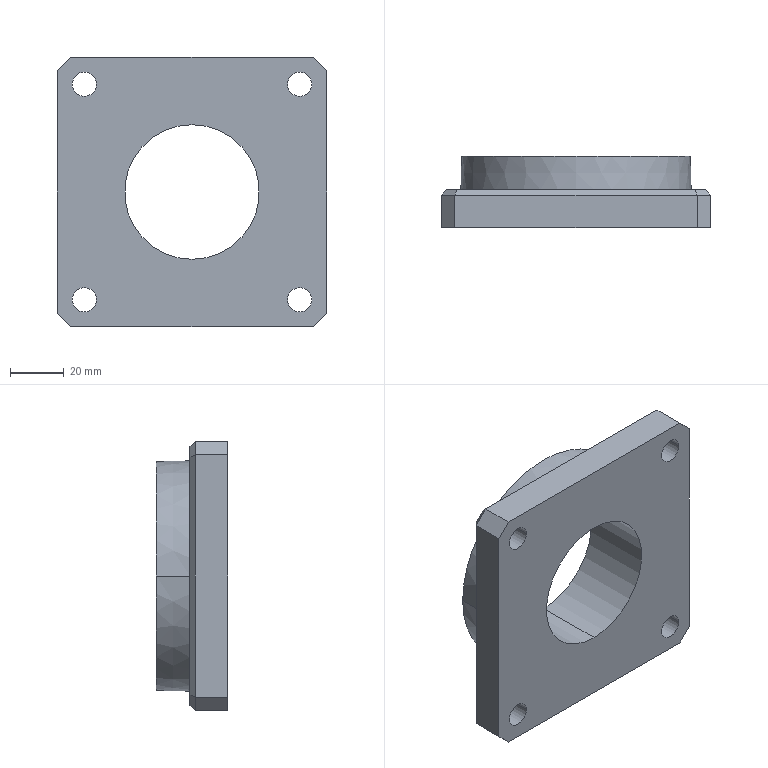Part | SolidWorks | features BaseBody 1 | 1 solid | 43 faces | box 100 x 26.5 x 100 mm | volume 151734 mm3 | plane 23 | cylinder 18 | cone 2 | commonest cylinder face diameters 9 x8 14 x8 50 x2
STEP:
#1=CARTESIAN_POINT('',(66.,42.,40.));
#2=VERTEX_POINT('',#1);
#3=CARTESIAN_POINT('',(80.,42.,40.));
#4=VERTEX_POINT('',#3);
#5=CARTESIAN_POINT('',(73.,42.,40.));
#6=DIRECTION('',(0.,1.,0.));
#7=DIRECTION('',(-1.,0.,0.));
#8=AXIS2_PLACEMENT_3D('',#5,#6,#7);
#9=CIRCLE('',#8,7.);
#10=EDGE_CURVE('',#2,#4,#9,.T.);
#11=ORIENTED_EDGE('',*,*,#10,.F.);
#12=CARTESIAN_POINT('',(66.,49.,40.));
#13=VERTEX_POINT('',#12);
#14=CARTESIAN_POINT('',(66.,49.,40.));
#15=DIRECTION('',(0.,1.,0.));
#16=VECTOR('',#15,1000.);
#17=LINE('',#14,#16);
#18=EDGE_CURVE('',#2,#13,#17,.T.);
#19=ORIENTED_EDGE('',*,*,#18,.T.);
#20=CARTESIAN_POINT('',(80.,49.,40.));
#21=VERTEX_POINT('',#20);
#22=CARTESIAN_POINT('',(73.,49.,40.));
#23=DIRECTION('',(0.,-1.,0.));
#24=DIRECTION('',(1.,0.,0.));
#25=AXIS2_PLACEMENT_3D('',#22,#23,#24);
#26=CIRCLE('',#25,7.);
#27=EDGE_CURVE('',#21,#13,#26,.T.);
#28=ORIENTED_EDGE('',*,*,#27,.F.);
#29=CARTESIAN_POINT('',(80.,49.,40.));
#30=DIRECTION('',(0.,1.,0.));
#31=VECTOR('',#30,1000.);
#32=LINE('',#29,#31);
#33=EDGE_CURVE('',#4,#21,#32,.T.);
#34=ORIENTED_EDGE('',*,*,#33,.F.);
#35=EDGE_LOOP('',(#11,#19,#28,#34));
#36=FACE_OUTER_BOUND('',#35,.T.);
#37=CARTESIAN_POINT('',(73.,49.,40.));
#38=DIRECTION('',(0.,1.,0.));
#39=DIRECTION('',(1.,0.,0.));
#40=AXIS2_PLACEMENT_3D('',#37,#38,#39);
#41=CYLINDRICAL_SURFACE('',#40,7.);
#42=ADVANCED_FACE('',(#36),#41,.F.);
#43=CARTESIAN_POINT('',(77.5,42.,40.));
#44=VERTEX_POINT('',#43);
#45=CARTESIAN_POINT('',(68.5,42.,40.));
#46=VERTEX_POINT('',#45);
#47=CARTESIAN_POINT('',(73.,42.,40.));
#48=DIRECTION('',(0.,-1.,0.));
#49=DIRECTION('',(-1.,0.,0.));
#50=AXIS2_PLACEMENT_3D('',#47,#48,#49);
#51=CIRCLE('',#50,4.5);
#52=EDGE_CURVE('',#44,#46,#51,.T.);
#53=ORIENTED_EDGE('',*,*,#52,.F.);
#54=CARTESIAN_POINT('',(77.5,35.,40.));
#55=VERTEX_POINT('',#54);
#56=CARTESIAN_POINT('',(77.5,35.,40.));
#57=DIRECTION('',(0.,-1.,0.));
#58=VECTOR('',#57,1000.);
#59=LINE('',#56,#58);
#60=EDGE_CURVE('',#44,#55,#59,.T.);
#61=ORIENTED_EDGE('',*,*,#60,.T.);
#62=CARTESIAN_POINT('',(68.5,35.,40.));
#63=VERTEX_POINT('',#62);
#64=CARTESIAN_POINT('',(73.,35.,40.));
#65=DIRECTION('',(0.,1.,0.));
#66=DIRECTION('',(1.,0.,0.));
#67=AXIS2_PLACEMENT_3D('',#64,#65,#66);
#68=CIRCLE('',#67,4.5);
#69=EDGE_CURVE('',#63,#55,#68,.T.);
#70=ORIENTED_EDGE('',*,*,#69,.F.);
#71=CARTESIAN_POINT('',(68.5,35.,40.));
#72=DIRECTION('',(0.,-1.,0.));
#73=VECTOR('',#72,1000.);
#74=LINE('',#71,#73);
#75=EDGE_CURVE('',#46,#63,#74,.T.);
#76=ORIENTED_EDGE('',*,*,#75,.F.);
#77=EDGE_LOOP('',(#53,#61,#70,#76));
#78=FACE_OUTER_BOUND('',#77,.T.);
#79=CARTESIAN_POINT('',(73.,35.,40.));
#80=DIRECTION('',(0.,-1.,0.));
#81=DIRECTION('',(-1.,0.,0.));
#82=AXIS2_PLACEMENT_3D('',#79,#80,#81);
#83=CYLINDRICAL_SURFACE('',#82,4.5);
#84=ADVANCED_FACE('',(#78),#83,.F.);
#85=CARTESIAN_POINT('',(33.,61.5,25.));
#86=VERTEX_POINT('',#85);
#87=CARTESIAN_POINT('',(33.,61.5,-25.));
#88=VERTEX_POINT('',#87);
#89=CARTESIAN_POINT('',(33.,61.5,0.));
#90=DIRECTION('',(0.,-1.,0.));
#91=DIRECTION('',(0.,0.,1.));
#92=AXIS2_PLACEMENT_3D('',#89,#90,#91);
#93=CIRCLE('',#92,25.);
#94=EDGE_CURVE('',#86,#88,#93,.T.);
#95=ORIENTED_EDGE('',*,*,#94,.F.);
#96=CARTESIAN_POINT('',(33.,35.,25.));
#97=VERTEX_POINT('',#96);
#98=CARTESIAN_POINT('',(33.,35.,25.));
#99=DIRECTION('',(0.,-1.,0.));
#100=VECTOR('',#99,1000.);
#101=LINE('',#98,#100);
#102=EDGE_CURVE('',#86,#97,#101,.T.);
#103=ORIENTED_EDGE('',*,*,#102,.T.);
#104=CARTESIAN_POINT('',(33.,35.,-25.));
#105=VERTEX_POINT('',#104);
#106=CARTESIAN_POINT('',(33.,35.,0.));
#107=DIRECTION('',(0.,1.,0.));
#108=DIRECTION('',(0.,0.,1.));
#109=AXIS2_PLACEMENT_3D('',#106,#107,#108);
#110=CIRCLE('',#109,25.);
#111=EDGE_CURVE('',#105,#97,#110,.T.);
#112=ORIENTED_EDGE('',*,*,#111,.F.);
#113=CARTESIAN_POINT('',(33.,35.,-25.));
#114=DIRECTION('',(0.,-1.,0.));
#115=VECTOR('',#114,1000.);
#116=LINE('',#113,#115);
#117=EDGE_CURVE('',#88,#105,#116,.T.);
#118=ORIENTED_EDGE('',*,*,#117,.F.);
#119=EDGE_LOOP('',(#95,#103,#112,#118));
#120=FACE_OUTER_BOUND('',#119,.T.);
#121=CARTESIAN_POINT('',(33.,35.,0.));
#122=DIRECTION('',(0.,-1.,0.));
#123=DIRECTION('',(0.,0.,-1.));
#124=AXIS2_PLACEMENT_3D('',#121,#122,#123);
#125=CYLINDRICAL_SURFACE('',#124,25.);
#126=ADVANCED_FACE('',(#120),#125,.F.);
#127=CARTESIAN_POINT('',(-14.,42.,40.));
#128=VERTEX_POINT('',#127);
#129=CARTESIAN_POINT('',(0.,42.,40.));
#130=VERTEX_POINT('',#129);
#131=CARTESIAN_POINT('',(-7.,42.,40.));
#132=DIRECTION('',(0.,1.,0.));
#133=DIRECTION('',(-1.,0.,0.));
#134=AXIS2_PLACEMENT_3D('',#131,#132,#133);
#135=CIRCLE('',#134,7.);
#136=EDGE_CURVE('',#128,#130,#135,.T.);
#137=ORIENTED_EDGE('',*,*,#136,.F.);
#138=CARTESIAN_POINT('',(-14.,49.,40.));
#139=VERTEX_POINT('',#138);
#140=CARTESIAN_POINT('',(-14.,49.,40.));
#141=DIRECTION('',(0.,1.,0.));
#142=VECTOR('',#141,1000.);
#143=LINE('',#140,#142);
#144=EDGE_CURVE('',#128,#139,#143,.T.);
#145=ORIENTED_EDGE('',*,*,#144,.T.);
#146=CARTESIAN_POINT('',(0.,49.,40.));
#147=VERTEX_POINT('',#146);
#148=CARTESIAN_POINT('',(-7.,49.,40.));
#149=DIRECTION('',(0.,-1.,0.));
#150=DIRECTION('',(1.,0.,0.));
#151=AXIS2_PLACEMENT_3D('',#148,#149,#150);
#152=CIRCLE('',#151,7.);
#153=EDGE_CURVE('',#147,#139,#152,.T.);
#154=ORIENTED_EDGE('',*,*,#153,.F.);
#155=CARTESIAN_POINT('',(0.,49.,40.));
#156=DIRECTION('',(0.,1.,0.));
#157=VECTOR('',#156,1000.);
#158=LINE('',#155,#157);
#159=EDGE_CURVE('',#130,#147,#158,.T.);
#160=ORIENTED_EDGE('',*,*,#159,.F.);
#161=EDGE_LOOP('',(#137,#145,#154,#160));
#162=FACE_OUTER_BOUND('',#161,.T.);
#163=CARTESIAN_POINT('',(-7.,49.,40.));
#164=DIRECTION('',(0.,1.,0.));
#165=DIRECTION('',(1.,0.,0.));
#166=AXIS2_PLACEMENT_3D('',#163,#164,#165);
#167=CYLINDRICAL_SURFACE('',#166,7.);
#168=ADVANCED_FACE('',(#162),#167,.F.);
#169=CARTESIAN_POINT('',(75.5,61.5,0.));
#170=VERTEX_POINT('',#169);
#171=CARTESIAN_POINT('',(-9.5,61.5,0.));
#172=VERTEX_POINT('',#171);
#173=CARTESIAN_POINT('',(33.,61.5,0.));
#174=DIRECTION('',(0.,1.,0.));
#175=DIRECTION('',(-1.,0.,0.));
#176=AXIS2_PLACEMENT_3D('',#173,#174,#175);
#177=CIRCLE('',#176,42.5);
#178=EDGE_CURVE('',#170,#172,#177,.T.);
#179=ORIENTED_EDGE('',*,*,#178,.F.);
#180=CARTESIAN_POINT('',(75.736,49.,0.));
#181=VERTEX_POINT('',#180);
#182=CARTESIAN_POINT('',(34.,2261.,0.));
#183=DIRECTION('',(0.01886,-0.9998,0.));
#184=VECTOR('',#183,1000.);
#185=LINE('',#182,#184);
#186=EDGE_CURVE('',#170,#181,#185,.T.);
#187=ORIENTED_EDGE('',*,*,#186,.T.);
#188=CARTESIAN_POINT('',(-9.736,49.,0.));
#189=VERTEX_POINT('',#188);
#190=CARTESIAN_POINT('',(33.,49.,0.));
#191=DIRECTION('',(0.,-1.,0.));
#192=DIRECTION('',(1.,0.,0.));
#193=AXIS2_PLACEMENT_3D('',#190,#191,#192);
#194=CIRCLE('',#193,42.736);
#195=EDGE_CURVE('',#189,#181,#194,.T.);
#196=ORIENTED_EDGE('',*,*,#195,.F.);
#197=CARTESIAN_POINT('',(32.,2261.,0.));
#198=DIRECTION('',(-0.01886,-0.9998,0.));
#199=VECTOR('',#198,1000.);
#200=LINE('',#197,#199);
#201=EDGE_CURVE('',#172,#189,#200,.T.);
#202=ORIENTED_EDGE('',*,*,#201,.F.);
#203=EDGE_LOOP('',(#179,#187,#196,#202));
#204=FACE_OUTER_BOUND('',#203,.T.);
#205=CARTESIAN_POINT('',(33.,2261.,0.));
#206=DIRECTION('',(0.,-1.,0.));
#207=DIRECTION('',(-1.,0.,0.));
#208=AXIS2_PLACEMENT_3D('',#205,#206,#207);
#209=CONICAL_SURFACE('',#208,1.,0.01887);
#210=ADVANCED_FACE('',(#204),#209,.T.);
#211=CARTESIAN_POINT('',(-2.5,42.,40.));
#212=VERTEX_POINT('',#211);
#213=CARTESIAN_POINT('',(-11.5,42.,40.));
#214=VERTEX_POINT('',#213);
#215=CARTESIAN_POINT('',(-7.,42.,40.));
#216=DIRECTION('',(0.,-1.,0.));
#217=DIRECTION('',(-1.,0.,0.));
#218=AXIS2_PLACEMENT_3D('',#215,#216,#217);
#219=CIRCLE('',#218,4.5);
#220=EDGE_CURVE('',#212,#214,#219,.T.);
#221=ORIENTED_EDGE('',*,*,#220,.F.);
#222=CARTESIAN_POINT('',(-2.5,35.,40.));
#223=VERTEX_POINT('',#222);
#224=CARTESIAN_POINT('',(-2.5,35.,40.));
#225=DIRECTION('',(0.,-1.,0.));
#226=VECTOR('',#225,1000.);
#227=LINE('',#224,#226);
#228=EDGE_CURVE('',#212,#223,#227,.T.);
#229=ORIENTED_EDGE('',*,*,#228,.T.);
#230=CARTESIAN_POINT('',(-11.5,35.,40.));
#231=VERTEX_POINT('',#230);
#232=CARTESIAN_POINT('',(-7.,35.,40.));
#233=DIRECTION('',(0.,1.,0.));
#234=DIRECTION('',(-1.,0.,0.));
#235=AXIS2_PLACEMENT_3D('',#232,#233,#234);
#236=CIRCLE('',#235,4.5);
#237=EDGE_CURVE('',#231,#223,#236,.T.);
#238=ORIENTED_EDGE('',*,*,#237,.F.);
#239=CARTESIAN_POINT('',(-11.5,35.,40.));
#240=DIRECTION('',(0.,-1.,0.));
#241=VECTOR('',#240,1000.);
#242=LINE('',#239,#241);
#243=EDGE_CURVE('',#214,#231,#242,.T.);
#244=ORIENTED_EDGE('',*,*,#243,.F.);
#245=EDGE_LOOP('',(#221,#229,#238,#244));
#246=FACE_OUTER_BOUND('',#245,.T.);
#247=CARTESIAN_POINT('',(-7.,35.,40.));
#248=DIRECTION('',(0.,-1.,0.));
#249=DIRECTION('',(-1.,0.,0.));
#250=AXIS2_PLACEMENT_3D('',#247,#248,#249);
#251=CYLINDRICAL_SURFACE('',#250,4.5);
#252=ADVANCED_FACE('',(#246),#251,.F.);
#253=CARTESIAN_POINT('',(77.5,42.,-40.));
#254=VERTEX_POINT('',#253);
#255=CARTESIAN_POINT('',(68.5,42.,-40.));
#256=VERTEX_POINT('',#255);
#257=CARTESIAN_POINT('',(73.,42.,-40.));
#258=DIRECTION('',(0.,-1.,0.));
#259=DIRECTION('',(-1.,0.,0.));
#260=AXIS2_PLACEMENT_3D('',#257,#258,#259);
#261=CIRCLE('',#260,4.5);
#262=EDGE_CURVE('',#254,#256,#261,.T.);
#263=ORIENTED_EDGE('',*,*,#262,.F.);
#264=CARTESIAN_POINT('',(77.5,35.,-40.));
#265=VERTEX_POINT('',#264);
#266=CARTESIAN_POINT('',(77.5,35.,-40.));
#267=DIRECTION('',(0.,-1.,0.));
#268=VECTOR('',#267,1000.);
#269=LINE('',#266,#268);
#270=EDGE_CURVE('',#254,#265,#269,.T.);
#271=ORIENTED_EDGE('',*,*,#270,.T.);
#272=CARTESIAN_POINT('',(68.5,35.,-40.));
#273=VERTEX_POINT('',#272);
#274=CARTESIAN_POINT('',(73.,35.,-40.));
#275=DIRECTION('',(0.,1.,0.));
#276=DIRECTION('',(-1.,0.,0.));
#277=AXIS2_PLACEMENT_3D('',#274,#275,#276);
#278=CIRCLE('',#277,4.5);
#279=EDGE_CURVE('',#273,#265,#278,.T.);
#280=ORIENTED_EDGE('',*,*,#279,.F.);
#281=CARTESIAN_POINT('',(68.5,35.,-40.));
#282=DIRECTION('',(0.,-1.,0.));
#283=VECTOR('',#282,1000.);
#284=LINE('',#281,#283);
#285=EDGE_CURVE('',#256,#273,#284,.T.);
#286=ORIENTED_EDGE('',*,*,#285,.F.);
#287=EDGE_LOOP('',(#263,#271,#280,#286));
#288=FACE_OUTER_BOUND('',#287,.T.);
#289=CARTESIAN_POINT('',(73.,35.,-40.));
#290=DIRECTION('',(0.,-1.,0.));
#291=DIRECTION('',(-1.,0.,0.));
#292=AXIS2_PLACEMENT_3D('',#289,#290,#291);
#293=CYLINDRICAL_SURFACE('',#292,4.5);
#294=ADVANCED_FACE('',(#288),#293,.F.);
#295=CARTESIAN_POINT('',(-14.,42.,-40.));
#296=VERTEX_POINT('',#295);
#297=CARTESIAN_POINT('',(0.,42.,-40.));
#298=VERTEX_POINT('',#297);
#299=CARTESIAN_POINT('',(-7.,42.,-40.));
#300=DIRECTION('',(0.,1.,0.));
#301=DIRECTION('',(-1.,0.,0.));
#302=AXIS2_PLACEMENT_3D('',#299,#300,#301);
#303=CIRCLE('',#302,7.);
#304=EDGE_CURVE('',#296,#298,#303,.T.);
#305=ORIENTED_EDGE('',*,*,#304,.F.);
#306=CARTESIAN_POINT('',(-14.,49.,-40.));
#307=VERTEX_POINT('',#306);
#308=CARTESIAN_POINT('',(-14.,49.,-40.));
#309=DIRECTION('',(0.,1.,0.));
#310=VECTOR('',#309,1000.);
#311=LINE('',#308,#310);
#312=EDGE_CURVE('',#296,#307,#311,.T.);
#313=ORIENTED_EDGE('',*,*,#312,.T.);
#314=CARTESIAN_POINT('',(0.,49.,-40.));
#315=VERTEX_POINT('',#314);
#316=CARTESIAN_POINT('',(-7.,49.,-40.));
#317=DIRECTION('',(0.,-1.,0.));
#318=DIRECTION('',(1.,0.,0.));
#319=AXIS2_PLACEMENT_3D('',#316,#317,#318);
#320=CIRCLE('',#319,7.);
#321=EDGE_CURVE('',#315,#307,#320,.T.);
#322=ORIENTED_EDGE('',*,*,#321,.F.);
#323=CARTESIAN_POINT('',(0.,49.,-40.));
#324=DIRECTION('',(0.,1.,0.));
#325=VECTOR('',#324,1000.);
#326=LINE('',#323,#325);
#327=EDGE_CURVE('',#298,#315,#326,.T.);
#328=ORIENTED_EDGE('',*,*,#327,.F.);
#329=EDGE_LOOP('',(#305,#313,#322,#328));
#330=FACE_OUTER_BOUND('',#329,.T.);
#331=CARTESIAN_POINT('',(-7.,49.,-40.));
#332=DIRECTION('',(0.,1.,0.));
#333=DIRECTION('',(1.,0.,0.));
#334=AXIS2_PLACEMENT_3D('',#331,#332,#333);
#335=CYLINDRICAL_SURFACE('',#334,7.);
#336=ADVANCED_FACE('',(#330),#335,.F.);
#337=CARTESIAN_POINT('',(-2.5,42.,-40.));
#338=VERTEX_POINT('',#337);
#339=CARTESIAN_POINT('',(-11.5,42.,-40.));
#340=VERTEX_POINT('',#339);
#341=CARTESIAN_POINT('',(-7.,42.,-40.));
#342=DIRECTION('',(0.,-1.,0.));
#343=DIRECTION('',(-1.,0.,0.));
#344=AXIS2_PLACEMENT_3D('',#341,#342,#343);
#345=CIRCLE('',#344,4.5);
#346=EDGE_CURVE('',#338,#340,#345,.T.);
#347=ORIENTED_EDGE('',*,*,#346,.F.);
#348=CARTESIAN_POINT('',(-2.5,35.,-40.));
#349=VERTEX_POINT('',#348);
#350=CARTESIAN_POINT('',(-2.5,35.,-40.));
#351=DIRECTION('',(0.,-1.,0.));
#352=VECTOR('',#351,1000.);
#353=LINE('',#350,#352);
#354=EDGE_CURVE('',#338,#349,#353,.T.);
#355=ORIENTED_EDGE('',*,*,#354,.T.);
#356=CARTESIAN_POINT('',(-11.5,35.,-40.));
#357=VERTEX_POINT('',#356);
#358=CARTESIAN_POINT('',(-7.,35.,-40.));
#359=DIRECTION('',(0.,1.,0.));
#360=DIRECTION('',(1.,0.,0.));
#361=AXIS2_PLACEMENT_3D('',#358,#359,#360);
#362=CIRCLE('',#361,4.5);
#363=EDGE_CURVE('',#357,#349,#362,.T.);
#364=ORIENTED_EDGE('',*,*,#363,.F.);
#365=CARTESIAN_POINT('',(-11.5,35.,-40.));
#366=DIRECTION('',(0.,-1.,0.));
#367=VECTOR('',#366,1000.);
#368=LINE('',#365,#367);
#369=EDGE_CURVE('',#340,#357,#368,.T.);
#370=ORIENTED_EDGE('',*,*,#369,.F.);
#371=EDGE_LOOP('',(#347,#355,#364,#370));
#372=FACE_OUTER_BOUND('',#371,.T.);
#373=CARTESIAN_POINT('',(-7.,35.,-40.));
#374=DIRECTION('',(0.,-1.,0.));
#375=DIRECTION('',(-1.,0.,0.));
#376=AXIS2_PLACEMENT_3D('',#373,#374,#375);
#377=CYLINDRICAL_SURFACE('',#376,4.5);
#378=ADVANCED_FACE('',(#372),#377,.F.);
#379=CARTESIAN_POINT('',(66.,42.,-40.));
#380=VERTEX_POINT('',#379);
#381=CARTESIAN_POINT('',(80.,42.,-40.));
#382=VERTEX_POINT('',#381);
#383=CARTESIAN_POINT('',(73.,42.,-40.));
#384=DIRECTION('',(0.,1.,0.));
#385=DIRECTION('',(-1.,0.,0.));
#386=AXIS2_PLACEMENT_3D('',#383,#384,#385);
#387=CIRCLE('',#386,7.);
#388=EDGE_CURVE('',#380,#382,#387,.T.);
#389=ORIENTED_EDGE('',*,*,#388,.F.);
#390=CARTESIAN_POINT('',(66.,49.,-40.));
#391=VERTEX_POINT('',#390);
#392=CARTESIAN_POINT('',(66.,49.,-40.));
#393=DIRECTION('',(0.,1.,0.));
#394=VECTOR('',#393,1000.);
#395=LINE('',#392,#394);
#396=EDGE_CURVE('',#380,#391,#395,.T.);
#397=ORIENTED_EDGE('',*,*,#396,.T.);
#398=CARTESIAN_POINT('',(80.,49.,-40.));
#399=VERTEX_POINT('',#398);
#400=CARTESIAN_POINT('',(73.,49.,-40.));
#401=DIRECTION('',(0.,-1.,0.));
#402=DIRECTION('',(1.,0.,0.));
#403=AXIS2_PLACEMENT_3D('',#400,#401,#402);
#404=CIRCLE('',#403,7.);
#405=EDGE_CURVE('',#399,#391,#404,.T.);
#406=ORIENTED_EDGE('',*,*,#405,.F.);
#407=CARTESIAN_POINT('',(80.,49.,-40.));
#408=DIRECTION('',(0.,1.,0.));
#409=VECTOR('',#408,1000.);
#410=LINE('',#407,#409);
#411=EDGE_CURVE('',#382,#399,#410,.T.);
#412=ORIENTED_EDGE('',*,*,#411,.F.);
#413=EDGE_LOOP('',(#389,#397,#406,#412));
#414=FACE_OUTER_BOUND('',#413,.T.);
#415=CARTESIAN_POINT('',(73.,49.,-40.));
#416=DIRECTION('',(0.,1.,0.));
#417=DIRECTION('',(1.,0.,0.));
#418=AXIS2_PLACEMENT_3D('',#415,#416,#417);
#419=CYLINDRICAL_SURFACE('',#418,7.);
#420=ADVANCED_FACE('',(#414),#419,.F.);
#421=ORIENTED_EDGE('',*,*,#396,.F.);
#422=CARTESIAN_POINT('',(73.,42.,-40.));
#423=DIRECTION('',(0.,1.,0.));
#424=DIRECTION('',(-1.,0.,0.));
#425=AXIS2_PLACEMENT_3D('',#422,#423,#424);
#426=CIRCLE('',#425,7.);
#427=EDGE_CURVE('',#382,#380,#426,.T.);
#428=ORIENTED_EDGE('',*,*,#427,.F.);
#429=ORIENTED_EDGE('',*,*,#411,.T.);
#430=CARTESIAN_POINT('',(73.,49.,-40.));
#431=DIRECTION('',(0.,-1.,0.));
#432=DIRECTION('',(1.,0.,0.));
#433=AXIS2_PLACEMENT_3D('',#430,#431,#432);
#434=CIRCLE('',#433,7.);
#435=EDGE_CURVE('',#391,#399,#434,.T.);
#436=ORIENTED_EDGE('',*,*,#435,.F.);
#437=EDGE_LOOP('',(#421,#428,#429,#436));
#438=FACE_OUTER_BOUND('',#437,.T.);
#439=CARTESIAN_POINT('',(73.,49.,-40.));
#440=DIRECTION('',(0.,1.,0.));
#441=DIRECTION('',(1.,0.,0.));
#442=AXIS2_PLACEMENT_3D('',#439,#440,#441);
#443=CYLINDRICAL_SURFACE('',#442,7.);
#444=ADVANCED_FACE('',(#438),#443,.F.);
#445=ORIENTED_EDGE('',*,*,#354,.F.);
#446=CARTESIAN_POINT('',(-7.,42.,-40.));
#447=DIRECTION('',(0.,-1.,0.));
#448=DIRECTION('',(-1.,0.,0.));
#449=AXIS2_PLACEMENT_3D('',#446,#447,#448);
#450=CIRCLE('',#449,4.5);
#451=EDGE_CURVE('',#340,#338,#450,.T.);
#452=ORIENTED_EDGE('',*,*,#451,.F.);
#453=ORIENTED_EDGE('',*,*,#369,.T.);
#454=CARTESIAN_POINT('',(-7.,35.,-40.));
#455=DIRECTION('',(0.,1.,0.));
#456=DIRECTION('',(1.,0.,0.));
#457=AXIS2_PLACEMENT_3D('',#454,#455,#456);
#458=CIRCLE('',#457,4.5);
#459=EDGE_CURVE('',#349,#357,#458,.T.);
#460=ORIENTED_EDGE('',*,*,#459,.F.);
#461=EDGE_LOOP('',(#445,#452,#453,#460));
#462=FACE_OUTER_BOUND('',#461,.T.);
#463=CARTESIAN_POINT('',(-7.,35.,-40.));
#464=DIRECTION('',(0.,-1.,0.));
#465=DIRECTION('',(-1.,0.,0.));
#466=AXIS2_PLACEMENT_3D('',#463,#464,#465);
#467=CYLINDRICAL_SURFACE('',#466,4.5);
#468=ADVANCED_FACE('',(#462),#467,.F.);
#469=CARTESIAN_POINT('',(73.,42.,-40.));
#470=DIRECTION('',(0.,-1.,0.));
#471=DIRECTION('',(-1.,0.,0.));
#472=AXIS2_PLACEMENT_3D('',#469,#470,#471);
#473=CIRCLE('',#472,4.5);
#474=EDGE_CURVE('',#256,#254,#473,.T.);
#475=ORIENTED_EDGE('',*,*,#474,.T.);
#476=ORIENTED_EDGE('',*,*,#262,.T.);
#477=EDGE_LOOP('',(#475,#476));
#478=FACE_BOUND('',#477,.T.);
#479=ORIENTED_EDGE('',*,*,#427,.T.);
#480=ORIENTED_EDGE('',*,*,#388,.T.);
#481=EDGE_LOOP('',(#479,#480));
#482=FACE_OUTER_BOUND('',#481,.T.);
#483=CARTESIAN_POINT('',(79.368,42.,0.));
#484=DIRECTION('',(0.,1.,0.));
#485=DIRECTION('',(1.,0.,0.));
#486=AXIS2_PLACEMENT_3D('',#483,#484,#485);
#487=PLANE('',#486);
#488=ADVANCED_FACE('',(#478,#482),#487,.T.);
#489=ORIENTED_EDGE('',*,*,#451,.T.);
#490=ORIENTED_EDGE('',*,*,#346,.T.);
#491=EDGE_LOOP('',(#489,#490));
#492=FACE_BOUND('',#491,.T.);
#493=CARTESIAN_POINT('',(-7.,42.,-40.));
#494=DIRECTION('',(0.,1.,0.));
#495=DIRECTION('',(-1.,0.,0.));
#496=AXIS2_PLACEMENT_3D('',#493,#494,#495);
#497=CIRCLE('',#496,7.);
#498=EDGE_CURVE('',#298,#296,#497,.T.);
#499=ORIENTED_EDGE('',*,*,#498,.T.);
#500=ORIENTED_EDGE('',*,*,#304,.T.);
#501=EDGE_LOOP('',(#499,#500));
#502=FACE_OUTER_BOUND('',#501,.T.);
#503=CARTESIAN_POINT('',(79.368,42.,0.));
#504=DIRECTION('',(0.,1.,0.));
#505=DIRECTION('',(1.,0.,0.));
#506=AXIS2_PLACEMENT_3D('',#503,#504,#505);
#507=PLANE('',#506);
#508=ADVANCED_FACE('',(#492,#502),#507,.T.);
#509=ORIENTED_EDGE('',*,*,#312,.F.);
#510=ORIENTED_EDGE('',*,*,#498,.F.);
#511=ORIENTED_EDGE('',*,*,#327,.T.);
#512=CARTESIAN_POINT('',(-7.,49.,-40.));
#513=DIRECTION('',(0.,-1.,0.));
#514=DIRECTION('',(1.,0.,0.));
#515=AXIS2_PLACEMENT_3D('',#512,#513,#514);
#516=CIRCLE('',#515,7.);
#517=EDGE_CURVE('',#307,#315,#516,.T.);
#518=ORIENTED_EDGE('',*,*,#517,.F.);
#519=EDGE_LOOP('',(#509,#510,#511,#518));
#520=FACE_OUTER_BOUND('',#519,.T.);
#521=CARTESIAN_POINT('',(-7.,49.,-40.));
#522=DIRECTION('',(0.,1.,0.));
#523=DIRECTION('',(1.,0.,0.));
#524=AXIS2_PLACEMENT_3D('',#521,#522,#523);
#525=CYLINDRICAL_SURFACE('',#524,7.);
#526=ADVANCED_FACE('',(#520),#525,.F.);
#527=ORIENTED_EDGE('',*,*,#270,.F.);
#528=ORIENTED_EDGE('',*,*,#474,.F.);
#529=ORIENTED_EDGE('',*,*,#285,.T.);
#530=CARTESIAN_POINT('',(73.,35.,-40.));
#531=DIRECTION('',(0.,1.,0.));
#532=DIRECTION('',(-1.,0.,0.));
#533=AXIS2_PLACEMENT_3D('',#530,#531,#532);
#534=CIRCLE('',#533,4.5);
#535=EDGE_CURVE('',#265,#273,#534,.T.);
#536=ORIENTED_EDGE('',*,*,#535,.F.);
#537=EDGE_LOOP('',(#527,#528,#529,#536));
#538=FACE_OUTER_BOUND('',#537,.T.);
#539=CARTESIAN_POINT('',(73.,35.,-40.));
#540=DIRECTION('',(0.,-1.,0.));
#541=DIRECTION('',(-1.,0.,0.));
#542=AXIS2_PLACEMENT_3D('',#539,#540,#541);
#543=CYLINDRICAL_SURFACE('',#542,4.5);
#544=ADVANCED_FACE('',(#538),#543,.F.);
#545=ORIENTED_EDGE('',*,*,#228,.F.);
#546=CARTESIAN_POINT('',(-7.,42.,40.));
#547=DIRECTION('',(0.,-1.,0.));
#548=DIRECTION('',(-1.,0.,0.));
#549=AXIS2_PLACEMENT_3D('',#546,#547,#548);
#550=CIRCLE('',#549,4.5);
#551=EDGE_CURVE('',#214,#212,#550,.T.);
#552=ORIENTED_EDGE('',*,*,#551,.F.);
#553=ORIENTED_EDGE('',*,*,#243,.T.);
#554=CARTESIAN_POINT('',(-7.,35.,40.));
#555=DIRECTION('',(0.,1.,0.));
#556=DIRECTION('',(-1.,0.,0.));
#557=AXIS2_PLACEMENT_3D('',#554,#555,#556);
#558=CIRCLE('',#557,4.5);
#559=EDGE_CURVE('',#223,#231,#558,.T.);
#560=ORIENTED_EDGE('',*,*,#559,.F.);
#561=EDGE_LOOP('',(#545,#552,#553,#560));
#562=FACE_OUTER_BOUND('',#561,.T.);
#563=CARTESIAN_POINT('',(-7.,35.,40.));
#564=DIRECTION('',(0.,-1.,0.));
#565=DIRECTION('',(-1.,0.,0.));
#566=AXIS2_PLACEMENT_3D('',#563,#564,#565);
#567=CYLINDRICAL_SURFACE('',#566,4.5);
#568=ADVANCED_FACE('',(#562),#567,.F.);
#569=ORIENTED_EDGE('',*,*,#551,.T.);
#570=ORIENTED_EDGE('',*,*,#220,.T.);
#571=EDGE_LOOP('',(#569,#570));
#572=FACE_BOUND('',#571,.T.);
#573=CARTESIAN_POINT('',(-7.,42.,40.));
#574=DIRECTION('',(0.,1.,0.));
#575=DIRECTION('',(-1.,0.,0.));
#576=AXIS2_PLACEMENT_3D('',#573,#574,#575);
#577=CIRCLE('',#576,7.);
#578=EDGE_CURVE('',#130,#128,#577,.T.);
#579=ORIENTED_EDGE('',*,*,#578,.T.);
#580=ORIENTED_EDGE('',*,*,#136,.T.);
#581=EDGE_LOOP('',(#579,#580));
#582=FACE_OUTER_BOUND('',#581,.T.);
#583=CARTESIAN_POINT('',(79.368,42.,0.));
#584=DIRECTION('',(0.,1.,0.));
#585=DIRECTION('',(1.,0.,0.));
#586=AXIS2_PLACEMENT_3D('',#583,#584,#585);
#587=PLANE('',#586);
#588=ADVANCED_FACE('',(#572,#582),#587,.T.);
#589=ORIENTED_EDGE('',*,*,#186,.F.);
#590=CARTESIAN_POINT('',(33.,61.5,0.));
#591=DIRECTION('',(0.,1.,0.));
#592=DIRECTION('',(-1.,0.,0.));
#593=AXIS2_PLACEMENT_3D('',#590,#591,#592);
#594=CIRCLE('',#593,42.5);
#595=EDGE_CURVE('',#172,#170,#594,.T.);
#596=ORIENTED_EDGE('',*,*,#595,.F.);
#597=ORIENTED_EDGE('',*,*,#201,.T.);
#598=CARTESIAN_POINT('',(33.,49.,0.));
#599=DIRECTION('',(0.,-1.,0.));
#600=DIRECTION('',(1.,0.,0.));
#601=AXIS2_PLACEMENT_3D('',#598,#599,#600);
#602=CIRCLE('',#601,42.736);
#603=EDGE_CURVE('',#181,#189,#602,.T.);
#604=ORIENTED_EDGE('',*,*,#603,.F.);
#605=EDGE_LOOP('',(#589,#596,#597,#604));
#606=FACE_OUTER_BOUND('',#605,.T.);
#607=CARTESIAN_POINT('',(33.,2261.,0.));
#608=DIRECTION('',(0.,-1.,0.));
#609=DIRECTION('',(-1.,0.,0.));
#610=AXIS2_PLACEMENT_3D('',#607,#608,#609);
#611=CONICAL_SURFACE('',#610,1.,0.01887);
#612=ADVANCED_FACE('',(#606),#611,.T.);
#613=ORIENTED_EDGE('',*,*,#144,.F.);
#614=ORIENTED_EDGE('',*,*,#578,.F.);
#615=ORIENTED_EDGE('',*,*,#159,.T.);
#616=CARTESIAN_POINT('',(-7.,49.,40.));
#617=DIRECTION('',(0.,-1.,0.));
#618=DIRECTION('',(1.,0.,0.));
#619=AXIS2_PLACEMENT_3D('',#616,#617,#618);
#620=CIRCLE('',#619,7.);
#621=EDGE_CURVE('',#139,#147,#620,.T.);
#622=ORIENTED_EDGE('',*,*,#621,.F.);
#623=EDGE_LOOP('',(#613,#614,#615,#622));
#624=FACE_OUTER_BOUND('',#623,.T.);
#625=CARTESIAN_POINT('',(-7.,49.,40.));
#626=DIRECTION('',(0.,1.,0.));
#627=DIRECTION('',(1.,0.,0.));
#628=AXIS2_PLACEMENT_3D('',#625,#626,#627);
#629=CYLINDRICAL_SURFACE('',#628,7.);
#630=ADVANCED_FACE('',(#624),#629,.F.);
#631=ORIENTED_EDGE('',*,*,#102,.F.);
#632=CARTESIAN_POINT('',(33.,61.5,0.));
#633=DIRECTION('',(0.,-1.,0.));
#634=DIRECTION('',(0.,0.,1.));
#635=AXIS2_PLACEMENT_3D('',#632,#633,#634);
#636=CIRCLE('',#635,25.);
#637=EDGE_CURVE('',#88,#86,#636,.T.);
#638=ORIENTED_EDGE('',*,*,#637,.F.);
#639=ORIENTED_EDGE('',*,*,#117,.T.);
#640=CARTESIAN_POINT('',(33.,35.,0.));
#641=DIRECTION('',(0.,1.,0.));
#642=DIRECTION('',(0.,0.,1.));
#643=AXIS2_PLACEMENT_3D('',#640,#641,#642);
#644=CIRCLE('',#643,25.);
#645=EDGE_CURVE('',#97,#105,#644,.T.);
#646=ORIENTED_EDGE('',*,*,#645,.F.);
#647=EDGE_LOOP('',(#631,#638,#639,#646));
#648=FACE_OUTER_BOUND('',#647,.T.);
#649=CARTESIAN_POINT('',(33.,35.,0.));
#650=DIRECTION('',(0.,-1.,0.));
#651=DIRECTION('',(0.,0.,-1.));
#652=AXIS2_PLACEMENT_3D('',#649,#650,#651);
#653=CYLINDRICAL_SURFACE('',#652,25.);
#654=ADVANCED_FACE('',(#648),#653,.F.);
#655=ORIENTED_EDGE('',*,*,#60,.F.);
#656=CARTESIAN_POINT('',(73.,42.,40.));
#657=DIRECTION('',(0.,-1.,0.));
#658=DIRECTION('',(-1.,0.,0.));
#659=AXIS2_PLACEMENT_3D('',#656,#657,#658);
#660=CIRCLE('',#659,4.5);
#661=EDGE_CURVE('',#46,#44,#660,.T.);
#662=ORIENTED_EDGE('',*,*,#661,.F.);
#663=ORIENTED_EDGE('',*,*,#75,.T.);
#664=CARTESIAN_POINT('',(73.,35.,40.));
#665=DIRECTION('',(0.,1.,0.));
#666=DIRECTION('',(1.,0.,0.));
#667=AXIS2_PLACEMENT_3D('',#664,#665,#666);
#668=CIRCLE('',#667,4.5);
#669=EDGE_CURVE('',#55,#63,#668,.T.);
#670=ORIENTED_EDGE('',*,*,#669,.F.);
#671=EDGE_LOOP('',(#655,#662,#663,#670));
#672=FACE_OUTER_BOUND('',#671,.T.);
#673=CARTESIAN_POINT('',(73.,35.,40.));
#674=DIRECTION('',(0.,-1.,0.));
#675=DIRECTION('',(-1.,0.,0.));
#676=AXIS2_PLACEMENT_3D('',#673,#674,#675);
#677=CYLINDRICAL_SURFACE('',#676,4.5);
#678=ADVANCED_FACE('',(#672),#677,.F.);
#679=ORIENTED_EDGE('',*,*,#637,.T.);
#680=ORIENTED_EDGE('',*,*,#94,.T.);
#681=EDGE_LOOP('',(#679,#680));
#682=FACE_BOUND('',#681,.T.);
#683=ORIENTED_EDGE('',*,*,#595,.T.);
#684=ORIENTED_EDGE('',*,*,#178,.T.);
#685=EDGE_LOOP('',(#683,#684));
#686=FACE_OUTER_BOUND('',#685,.T.);
#687=CARTESIAN_POINT('',(11.75,61.5,0.));
#688=DIRECTION('',(0.,1.,0.));
#689=DIRECTION('',(1.,0.,0.));
#690=AXIS2_PLACEMENT_3D('',#687,#688,#689);
#691=PLANE('',#690);
#692=ADVANCED_FACE('',(#682,#686),#691,.T.);
#693=ORIENTED_EDGE('',*,*,#661,.T.);
#694=ORIENTED_EDGE('',*,*,#52,.T.);
#695=EDGE_LOOP('',(#693,#694));
#696=FACE_BOUND('',#695,.T.);
#697=CARTESIAN_POINT('',(73.,42.,40.));
#698=DIRECTION('',(0.,1.,0.));
#699=DIRECTION('',(-1.,0.,0.));
#700=AXIS2_PLACEMENT_3D('',#697,#698,#699);
#701=CIRCLE('',#700,7.);
#702=EDGE_CURVE('',#4,#2,#701,.T.);
#703=ORIENTED_EDGE('',*,*,#702,.T.);
#704=ORIENTED_EDGE('',*,*,#10,.T.);
#705=EDGE_LOOP('',(#703,#704));
#706=FACE_OUTER_BOUND('',#705,.T.);
#707=CARTESIAN_POINT('',(79.368,42.,0.));
#708=DIRECTION('',(0.,1.,0.));
#709=DIRECTION('',(1.,0.,0.));
#710=AXIS2_PLACEMENT_3D('',#707,#708,#709);
#711=PLANE('',#710);
#712=ADVANCED_FACE('',(#696,#706),#711,.T.);
#713=ORIENTED_EDGE('',*,*,#18,.F.);
#714=ORIENTED_EDGE('',*,*,#702,.F.);
#715=ORIENTED_EDGE('',*,*,#33,.T.);
#716=CARTESIAN_POINT('',(73.,49.,40.));
#717=DIRECTION('',(0.,-1.,0.));
#718=DIRECTION('',(1.,0.,0.));
#719=AXIS2_PLACEMENT_3D('',#716,#717,#718);
#720=CIRCLE('',#719,7.);
#721=EDGE_CURVE('',#13,#21,#720,.T.);
#722=ORIENTED_EDGE('',*,*,#721,.F.);
#723=EDGE_LOOP('',(#713,#714,#715,#722));
#724=FACE_OUTER_BOUND('',#723,.T.);
#725=CARTESIAN_POINT('',(73.,49.,40.));
#726=DIRECTION('',(0.,1.,0.));
#727=DIRECTION('',(1.,0.,0.));
#728=AXIS2_PLACEMENT_3D('',#725,#726,#727);
#729=CYLINDRICAL_SURFACE('',#728,7.);
#730=ADVANCED_FACE('',(#724),#729,.F.);
#731=ORIENTED_EDGE('',*,*,#195,.T.);
#732=ORIENTED_EDGE('',*,*,#603,.T.);
#733=EDGE_LOOP('',(#731,#732));
#734=FACE_BOUND('',#733,.T.);
#735=ORIENTED_EDGE('',*,*,#405,.T.);
#736=ORIENTED_EDGE('',*,*,#435,.T.);
#737=EDGE_LOOP('',(#735,#736));
#738=FACE_BOUND('',#737,.T.);
#739=ORIENTED_EDGE('',*,*,#321,.T.);
#740=ORIENTED_EDGE('',*,*,#517,.T.);
#741=EDGE_LOOP('',(#739,#740));
#742=FACE_BOUND('',#741,.T.);
#743=ORIENTED_EDGE('',*,*,#153,.T.);
#744=ORIENTED_EDGE('',*,*,#621,.T.);
#745=EDGE_LOOP('',(#743,#744));
#746=FACE_BOUND('',#745,.T.);
#747=ORIENTED_EDGE('',*,*,#27,.T.);
#748=ORIENTED_EDGE('',*,*,#721,.T.);
#749=EDGE_LOOP('',(#747,#748));
#750=FACE_BOUND('',#749,.T.);
#751=CARTESIAN_POINT('',(81.,49.,44.172));
#752=VERTEX_POINT('',#751);
#753=CARTESIAN_POINT('',(81.,49.,-44.172));
#754=VERTEX_POINT('',#753);
#755=CARTESIAN_POINT('',(81.,49.,44.172));
#756=DIRECTION('',(0.,0.,-1.));
#757=VECTOR('',#756,1000.);
#758=LINE('',#755,#757);
#759=EDGE_CURVE('',#752,#754,#758,.T.);
#760=ORIENTED_EDGE('',*,*,#759,.T.);
#761=CARTESIAN_POINT('',(77.172,49.,-48.));
#762=VERTEX_POINT('',#761);
#763=CARTESIAN_POINT('',(81.,49.,-44.172));
#764=DIRECTION('',(-0.7071,0.,-0.7071));
#765=VECTOR('',#764,1000.);
#766=LINE('',#763,#765);
#767=EDGE_CURVE('',#754,#762,#766,.T.);
#768=ORIENTED_EDGE('',*,*,#767,.T.);
#769=CARTESIAN_POINT('',(-11.172,49.,-48.));
#770=VERTEX_POINT('',#769);
#771=CARTESIAN_POINT('',(77.172,49.,-48.));
#772=DIRECTION('',(-1.,0.,0.));
#773=VECTOR('',#772,1000.);
#774=LINE('',#771,#773);
#775=EDGE_CURVE('',#762,#770,#774,.T.);
#776=ORIENTED_EDGE('',*,*,#775,.T.);
#777=CARTESIAN_POINT('',(-15.,49.,-44.172));
#778=VERTEX_POINT('',#777);
#779=CARTESIAN_POINT('',(-11.172,49.,-48.));
#780=DIRECTION('',(-0.7071,0.,0.7071));
#781=VECTOR('',#780,1000.);
#782=LINE('',#779,#781);
#783=EDGE_CURVE('',#770,#778,#782,.T.);
#784=ORIENTED_EDGE('',*,*,#783,.T.);
#785=CARTESIAN_POINT('',(-15.,49.,44.172));
#786=VERTEX_POINT('',#785);
#787=CARTESIAN_POINT('',(-15.,49.,-44.172));
#788=DIRECTION('',(0.,0.,1.));
#789=VECTOR('',#788,1000.);
#790=LINE('',#787,#789);
#791=EDGE_CURVE('',#778,#786,#790,.T.);
#792=ORIENTED_EDGE('',*,*,#791,.T.);
#793=CARTESIAN_POINT('',(-11.172,49.,48.));
#794=VERTEX_POINT('',#793);
#795=CARTESIAN_POINT('',(-15.,49.,44.172));
#796=DIRECTION('',(0.7071,0.,0.7071));
#797=VECTOR('',#796,1000.);
#798=LINE('',#795,#797);
#799=EDGE_CURVE('',#786,#794,#798,.T.);
#800=ORIENTED_EDGE('',*,*,#799,.T.);
#801=CARTESIAN_POINT('',(77.172,49.,48.));
#802=VERTEX_POINT('',#801);
#803=CARTESIAN_POINT('',(-11.172,49.,48.));
#804=DIRECTION('',(1.,0.,0.));
#805=VECTOR('',#804,1000.);
#806=LINE('',#803,#805);
#807=EDGE_CURVE('',#794,#802,#806,.T.);
#808=ORIENTED_EDGE('',*,*,#807,.T.);
#809=CARTESIAN_POINT('',(77.172,49.,48.));
#810=DIRECTION('',(0.7071,0.,-0.7071));
#811=VECTOR('',#810,1000.);
#812=LINE('',#809,#811);
#813=EDGE_CURVE('',#802,#752,#812,.T.);
#814=ORIENTED_EDGE('',*,*,#813,.T.);
#815=EDGE_LOOP('',(#760,#768,#776,#784,#792,#800,#808,#814));
#816=FACE_OUTER_BOUND('',#815,.T.);
#817=CARTESIAN_POINT('',(-1.,49.,0.));
#818=DIRECTION('',(0.,-1.,0.));
#819=DIRECTION('',(0.,0.,-1.));
#820=AXIS2_PLACEMENT_3D('',#817,#818,#819);
#821=PLANE('',#820);
#822=ADVANCED_FACE('',(#734,#738,#742,#746,#750,#816),#821,.F.);
#823=CARTESIAN_POINT('',(78.,47.,50.));
#824=VERTEX_POINT('',#823);
#825=CARTESIAN_POINT('',(83.,47.,45.));
#826=VERTEX_POINT('',#825);
#827=CARTESIAN_POINT('',(78.,47.,50.));
#828=DIRECTION('',(0.7071,0.,-0.7071));
#829=VECTOR('',#828,1000.);
#830=LINE('',#827,#829);
#831=EDGE_CURVE('',#824,#826,#830,.T.);
#832=ORIENTED_EDGE('',*,*,#831,.F.);
#833=CARTESIAN_POINT('',(78.,35.,50.));
#834=VERTEX_POINT('',#833);
#835=CARTESIAN_POINT('',(78.,35.,50.));
#836=DIRECTION('',(0.,1.,0.));
#837=VECTOR('',#836,1000.);
#838=LINE('',#835,#837);
#839=EDGE_CURVE('',#834,#824,#838,.T.);
#840=ORIENTED_EDGE('',*,*,#839,.F.);
#841=CARTESIAN_POINT('',(83.,35.,45.));
#842=VERTEX_POINT('',#841);
#843=CARTESIAN_POINT('',(83.,35.,45.));
#844=DIRECTION('',(-0.7071,0.,0.7071));
#845=VECTOR('',#844,1000.);
#846=LINE('',#843,#845);
#847=EDGE_CURVE('',#842,#834,#846,.T.);
#848=ORIENTED_EDGE('',*,*,#847,.F.);
#849=CARTESIAN_POINT('',(83.,35.,45.));
#850=DIRECTION('',(0.,1.,0.));
#851=VECTOR('',#850,1000.);
#852=LINE('',#849,#851);
#853=EDGE_CURVE('',#842,#826,#852,.T.);
#854=ORIENTED_EDGE('',*,*,#853,.T.);
#855=EDGE_LOOP('',(#832,#840,#848,#854));
#856=FACE_OUTER_BOUND('',#855,.T.);
#857=CARTESIAN_POINT('',(80.5,42.,47.5));
#858=DIRECTION('',(-0.7071,0.,-0.7071));
#859=DIRECTION('',(-0.7071,0.,0.7071));
#860=AXIS2_PLACEMENT_3D('',#857,#858,#859);
#861=PLANE('',#860);
#862=ADVANCED_FACE('',(#856),#861,.F.);
#863=ORIENTED_EDGE('',*,*,#831,.T.);
#864=CARTESIAN_POINT('',(81.,49.,44.172));
#865=DIRECTION('',(0.6786,-0.6786,0.2811));
#866=VECTOR('',#865,1000.);
#867=LINE('',#864,#866);
#868=EDGE_CURVE('',#752,#826,#867,.T.);
#869=ORIENTED_EDGE('',*,*,#868,.F.);
#870=ORIENTED_EDGE('',*,*,#813,.F.);
#871=CARTESIAN_POINT('',(77.172,49.,48.));
#872=DIRECTION('',(0.2811,-0.6786,0.6786));
#873=VECTOR('',#872,1000.);
#874=LINE('',#871,#873);
#875=EDGE_CURVE('',#802,#824,#874,.T.);
#876=ORIENTED_EDGE('',*,*,#875,.T.);
#877=EDGE_LOOP('',(#863,#869,#870,#876));
#878=FACE_OUTER_BOUND('',#877,.T.);
#879=CARTESIAN_POINT('',(78.793,48.,47.793));
#880=DIRECTION('',(0.5,0.7071,0.5));
#881=DIRECTION('',(0.7071,0.,-0.7071));
#882=AXIS2_PLACEMENT_3D('',#879,#880,#881);
#883=PLANE('',#882);
#884=ADVANCED_FACE('',(#878),#883,.T.);
#885=CARTESIAN_POINT('',(83.,47.,-45.));
#886=VERTEX_POINT('',#885);
#887=CARTESIAN_POINT('',(83.,47.,45.));
#888=DIRECTION('',(0.,0.,-1.));
#889=VECTOR('',#888,1000.);
#890=LINE('',#887,#889);
#891=EDGE_CURVE('',#826,#886,#890,.T.);
#892=ORIENTED_EDGE('',*,*,#891,.T.);
#893=CARTESIAN_POINT('',(81.,49.,-44.172));
#894=DIRECTION('',(0.6786,-0.6786,-0.2811));
#895=VECTOR('',#894,1000.);
#896=LINE('',#893,#895);
#897=EDGE_CURVE('',#754,#886,#896,.T.);
#898=ORIENTED_EDGE('',*,*,#897,.F.);
#899=ORIENTED_EDGE('',*,*,#759,.F.);
#900=ORIENTED_EDGE('',*,*,#868,.T.);
#901=EDGE_LOOP('',(#892,#898,#899,#900));
#902=FACE_OUTER_BOUND('',#901,.T.);
#903=CARTESIAN_POINT('',(82.,48.,1.414));
#904=DIRECTION('',(0.7071,0.7071,0.));
#905=DIRECTION('',(0.,0.,-1.));
#906=AXIS2_PLACEMENT_3D('',#903,#904,#905);
#907=PLANE('',#906);
#908=ADVANCED_FACE('',(#902),#907,.T.);
#909=ORIENTED_EDGE('',*,*,#891,.F.);
#910=ORIENTED_EDGE('',*,*,#853,.F.);
#911=CARTESIAN_POINT('',(83.,35.,-45.));
#912=VERTEX_POINT('',#911);
#913=CARTESIAN_POINT('',(83.,35.,45.));
#914=DIRECTION('',(0.,0.,-1.));
#915=VECTOR('',#914,1000.);
#916=LINE('',#913,#915);
#917=EDGE_CURVE('',#842,#912,#916,.T.);
#918=ORIENTED_EDGE('',*,*,#917,.T.);
#919=CARTESIAN_POINT('',(83.,35.,-45.));
#920=DIRECTION('',(0.,1.,0.));
#921=VECTOR('',#920,1000.);
#922=LINE('',#919,#921);
#923=EDGE_CURVE('',#912,#886,#922,.T.);
#924=ORIENTED_EDGE('',*,*,#923,.T.);
#925=EDGE_LOOP('',(#909,#910,#918,#924));
#926=FACE_OUTER_BOUND('',#925,.T.);
#927=CARTESIAN_POINT('',(83.,35.,50.));
#928=DIRECTION('',(-1.,0.,0.));
#929=DIRECTION('',(0.,0.,1.));
#930=AXIS2_PLACEMENT_3D('',#927,#928,#929);
#931=PLANE('',#930);
#932=ADVANCED_FACE('',(#926),#931,.F.);
#933=CARTESIAN_POINT('',(78.,47.,-50.));
#934=VERTEX_POINT('',#933);
#935=CARTESIAN_POINT('',(83.,47.,-45.));
#936=DIRECTION('',(-0.7071,0.,-0.7071));
#937=VECTOR('',#936,1000.);
#938=LINE('',#935,#937);
#939=EDGE_CURVE('',#886,#934,#938,.T.);
#940=ORIENTED_EDGE('',*,*,#939,.F.);
#941=ORIENTED_EDGE('',*,*,#923,.F.);
#942=CARTESIAN_POINT('',(78.,35.,-50.));
#943=VERTEX_POINT('',#942);
#944=CARTESIAN_POINT('',(78.,35.,-50.));
#945=DIRECTION('',(0.7071,0.,0.7071));
#946=VECTOR('',#945,1000.);
#947=LINE('',#944,#946);
#948=EDGE_CURVE('',#943,#912,#947,.T.);
#949=ORIENTED_EDGE('',*,*,#948,.F.);
#950=CARTESIAN_POINT('',(78.,35.,-50.));
#951=DIRECTION('',(0.,1.,0.));
#952=VECTOR('',#951,1000.);
#953=LINE('',#950,#952);
#954=EDGE_CURVE('',#943,#934,#953,.T.);
#955=ORIENTED_EDGE('',*,*,#954,.T.);
#956=EDGE_LOOP('',(#940,#941,#949,#955));
#957=FACE_OUTER_BOUND('',#956,.T.);
#958=CARTESIAN_POINT('',(80.5,42.,-47.5));
#959=DIRECTION('',(-0.7071,0.,0.7071));
#960=DIRECTION('',(0.,1.,0.));
#961=AXIS2_PLACEMENT_3D('',#958,#959,#960);
#962=PLANE('',#961);
#963=ADVANCED_FACE('',(#957),#962,.F.);
#964=ORIENTED_EDGE('',*,*,#939,.T.);
#965=CARTESIAN_POINT('',(77.172,49.,-48.));
#966=DIRECTION('',(0.2811,-0.6786,-0.6786));
#967=VECTOR('',#966,1000.);
#968=LINE('',#965,#967);
#969=EDGE_CURVE('',#762,#934,#968,.T.);
#970=ORIENTED_EDGE('',*,*,#969,.F.);
#971=ORIENTED_EDGE('',*,*,#767,.F.);
#972=ORIENTED_EDGE('',*,*,#897,.T.);
#973=EDGE_LOOP('',(#964,#970,#971,#972));
#974=FACE_OUTER_BOUND('',#973,.T.);
#975=CARTESIAN_POINT('',(80.793,48.,-45.793));
#976=DIRECTION('',(0.5,0.7071,-0.5));
#977=DIRECTION('',(-0.7071,0.,-0.7071));
#978=AXIS2_PLACEMENT_3D('',#975,#976,#977);
#979=PLANE('',#978);
#980=ADVANCED_FACE('',(#974),#979,.T.);
#981=CARTESIAN_POINT('',(-12.,47.,-50.));
#982=VERTEX_POINT('',#981);
#983=CARTESIAN_POINT('',(78.,47.,-50.));
#984=DIRECTION('',(-1.,0.,0.));
#985=VECTOR('',#984,1000.);
#986=LINE('',#983,#985);
#987=EDGE_CURVE('',#934,#982,#986,.T.);
#988=ORIENTED_EDGE('',*,*,#987,.T.);
#989=CARTESIAN_POINT('',(-12.,47.,-50.));
#990=DIRECTION('',(0.2811,0.6786,0.6786));
#991=VECTOR('',#990,1000.);
#992=LINE('',#989,#991);
#993=EDGE_CURVE('',#982,#770,#992,.T.);
#994=ORIENTED_EDGE('',*,*,#993,.T.);
#995=ORIENTED_EDGE('',*,*,#775,.F.);
#996=ORIENTED_EDGE('',*,*,#969,.T.);
#997=EDGE_LOOP('',(#988,#994,#995,#996));
#998=FACE_OUTER_BOUND('',#997,.T.);
#999=CARTESIAN_POINT('',(33.,48.,-49.));
#1000=DIRECTION('',(0.,0.7071,-0.7071));
#1001=DIRECTION('',(-1.,0.,0.));
#1002=AXIS2_PLACEMENT_3D('',#999,#1000,#1001);
#1003=PLANE('',#1002);
#1004=ADVANCED_FACE('',(#998),#1003,.T.);
#1005=ORIENTED_EDGE('',*,*,#987,.F.);
#1006=ORIENTED_EDGE('',*,*,#954,.F.);
#1007=CARTESIAN_POINT('',(-12.,35.,-50.));
#1008=VERTEX_POINT('',#1007);
#1009=CARTESIAN_POINT('',(78.,35.,-50.));
#1010=DIRECTION('',(-1.,0.,0.));
#1011=VECTOR('',#1010,1000.);
#1012=LINE('',#1009,#1011);
#1013=EDGE_CURVE('',#943,#1008,#1012,.T.);
#1014=ORIENTED_EDGE('',*,*,#1013,.T.);
#1015=CARTESIAN_POINT('',(-12.,35.,-50.));
#1016=DIRECTION('',(0.,1.,0.));
#1017=VECTOR('',#1016,1000.);
#1018=LINE('',#1015,#1017);
#1019=EDGE_CURVE('',#1008,#982,#1018,.T.);
#1020=ORIENTED_EDGE('',*,*,#1019,.T.);
#1021=EDGE_LOOP('',(#1005,#1006,#1014,#1020));
#1022=FACE_OUTER_BOUND('',#1021,.T.);
#1023=CARTESIAN_POINT('',(83.,35.,-50.));
#1024=DIRECTION('',(0.,0.,1.));
#1025=DIRECTION('',(1.,0.,0.));
#1026=AXIS2_PLACEMENT_3D('',#1023,#1024,#1025);
#1027=PLANE('',#1026);
#1028=ADVANCED_FACE('',(#1022),#1027,.F.);
#1029=CARTESIAN_POINT('',(-17.,47.,-45.));
#1030=VERTEX_POINT('',#1029);
#1031=CARTESIAN_POINT('',(-12.,47.,-50.));
#1032=DIRECTION('',(-0.7071,0.,0.7071));
#1033=VECTOR('',#1032,1000.);
#1034=LINE('',#1031,#1033);
#1035=EDGE_CURVE('',#982,#1030,#1034,.T.);
#1036=ORIENTED_EDGE('',*,*,#1035,.F.);
#1037=ORIENTED_EDGE('',*,*,#1019,.F.);
#1038=CARTESIAN_POINT('',(-17.,35.,-45.));
#1039=VERTEX_POINT('',#1038);
#1040=CARTESIAN_POINT('',(-17.,35.,-45.));
#1041=DIRECTION('',(0.7071,0.,-0.7071));
#1042=VECTOR('',#1041,1000.);
#1043=LINE('',#1040,#1042);
#1044=EDGE_CURVE('',#1039,#1008,#1043,.T.);
#1045=ORIENTED_EDGE('',*,*,#1044,.F.);
#1046=CARTESIAN_POINT('',(-17.,35.,-45.));
#1047=DIRECTION('',(0.,1.,0.));
#1048=VECTOR('',#1047,1000.);
#1049=LINE('',#1046,#1048);
#1050=EDGE_CURVE('',#1039,#1030,#1049,.T.);
#1051=ORIENTED_EDGE('',*,*,#1050,.T.);
#1052=EDGE_LOOP('',(#1036,#1037,#1045,#1051));
#1053=FACE_OUTER_BOUND('',#1052,.T.);
#1054=CARTESIAN_POINT('',(-14.5,42.,-47.5));
#1055=DIRECTION('',(0.7071,0.,0.7071));
#1056=DIRECTION('',(0.,-1.,0.));
#1057=AXIS2_PLACEMENT_3D('',#1054,#1055,#1056);
#1058=PLANE('',#1057);
#1059=ADVANCED_FACE('',(#1053),#1058,.F.);
#1060=ORIENTED_EDGE('',*,*,#1035,.T.);
#1061=CARTESIAN_POINT('',(-15.,49.,-44.172));
#1062=DIRECTION('',(-0.6786,-0.6786,-0.2811));
#1063=VECTOR('',#1062,1000.);
#1064=LINE('',#1061,#1063);
#1065=EDGE_CURVE('',#778,#1030,#1064,.T.);
#1066=ORIENTED_EDGE('',*,*,#1065,.F.);
#1067=ORIENTED_EDGE('',*,*,#783,.F.);
#1068=ORIENTED_EDGE('',*,*,#993,.F.);
#1069=EDGE_LOOP('',(#1060,#1066,#1067,#1068));
#1070=FACE_OUTER_BOUND('',#1069,.T.);
#1071=CARTESIAN_POINT('',(-13.793,48.,-46.793));
#1072=DIRECTION('',(-0.5,0.7071,-0.5));
#1073=DIRECTION('',(-0.7071,0.,0.7071));
#1074=AXIS2_PLACEMENT_3D('',#1071,#1072,#1073);
#1075=PLANE('',#1074);
#1076=ADVANCED_FACE('',(#1070),#1075,.T.);
#1077=CARTESIAN_POINT('',(-17.,47.,45.));
#1078=VERTEX_POINT('',#1077);
#1079=CARTESIAN_POINT('',(-17.,47.,-45.));
#1080=DIRECTION('',(0.,0.,1.));
#1081=VECTOR('',#1080,1000.);
#1082=LINE('',#1079,#1081);
#1083=EDGE_CURVE('',#1030,#1078,#1082,.T.);
#1084=ORIENTED_EDGE('',*,*,#1083,.T.);
#1085=CARTESIAN_POINT('',(-17.,47.,45.));
#1086=DIRECTION('',(0.6786,0.6786,-0.2811));
#1087=VECTOR('',#1086,1000.);
#1088=LINE('',#1085,#1087);
#1089=EDGE_CURVE('',#1078,#786,#1088,.T.);
#1090=ORIENTED_EDGE('',*,*,#1089,.T.);
#1091=ORIENTED_EDGE('',*,*,#791,.F.);
#1092=ORIENTED_EDGE('',*,*,#1065,.T.);
#1093=EDGE_LOOP('',(#1084,#1090,#1091,#1092));
#1094=FACE_OUTER_BOUND('',#1093,.T.);
#1095=CARTESIAN_POINT('',(-16.,48.,-1.414));
#1096=DIRECTION('',(-0.7071,0.7071,0.));
#1097=DIRECTION('',(0.,0.,1.));
#1098=AXIS2_PLACEMENT_3D('',#1095,#1096,#1097);
#1099=PLANE('',#1098);
#1100=ADVANCED_FACE('',(#1094),#1099,.T.);
#1101=ORIENTED_EDGE('',*,*,#1083,.F.);
#1102=ORIENTED_EDGE('',*,*,#1050,.F.);
#1103=CARTESIAN_POINT('',(-17.,35.,45.));
#1104=VERTEX_POINT('',#1103);
#1105=CARTESIAN_POINT('',(-17.,35.,-45.));
#1106=DIRECTION('',(0.,0.,1.));
#1107=VECTOR('',#1106,1000.);
#1108=LINE('',#1105,#1107);
#1109=EDGE_CURVE('',#1039,#1104,#1108,.T.);
#1110=ORIENTED_EDGE('',*,*,#1109,.T.);
#1111=CARTESIAN_POINT('',(-17.,35.,45.));
#1112=DIRECTION('',(0.,1.,0.));
#1113=VECTOR('',#1112,1000.);
#1114=LINE('',#1111,#1113);
#1115=EDGE_CURVE('',#1104,#1078,#1114,.T.);
#1116=ORIENTED_EDGE('',*,*,#1115,.T.);
#1117=EDGE_LOOP('',(#1101,#1102,#1110,#1116));
#1118=FACE_OUTER_BOUND('',#1117,.T.);
#1119=CARTESIAN_POINT('',(-17.,35.,-50.));
#1120=DIRECTION('',(1.,0.,0.));
#1121=DIRECTION('',(0.,1.,0.));
#1122=AXIS2_PLACEMENT_3D('',#1119,#1120,#1121);
#1123=PLANE('',#1122);
#1124=ADVANCED_FACE('',(#1118),#1123,.F.);
#1125=CARTESIAN_POINT('',(-12.,47.,50.));
#1126=VERTEX_POINT('',#1125);
#1127=CARTESIAN_POINT('',(-12.,47.,50.));
#1128=DIRECTION('',(-0.7071,0.,-0.7071));
#1129=VECTOR('',#1128,1000.);
#1130=LINE('',#1127,#1129);
#1131=EDGE_CURVE('',#1126,#1078,#1130,.T.);
#1132=ORIENTED_EDGE('',*,*,#1131,.T.);
#1133=ORIENTED_EDGE('',*,*,#1115,.F.);
#1134=CARTESIAN_POINT('',(-12.,35.,50.));
#1135=VERTEX_POINT('',#1134);
#1136=CARTESIAN_POINT('',(-12.,35.,50.));
#1137=DIRECTION('',(-0.7071,0.,-0.7071));
#1138=VECTOR('',#1137,1000.);
#1139=LINE('',#1136,#1138);
#1140=EDGE_CURVE('',#1135,#1104,#1139,.T.);
#1141=ORIENTED_EDGE('',*,*,#1140,.F.);
#1142=CARTESIAN_POINT('',(-12.,35.,50.));
#1143=DIRECTION('',(0.,1.,0.));
#1144=VECTOR('',#1143,1000.);
#1145=LINE('',#1142,#1144);
#1146=EDGE_CURVE('',#1135,#1126,#1145,.T.);
#1147=ORIENTED_EDGE('',*,*,#1146,.T.);
#1148=EDGE_LOOP('',(#1132,#1133,#1141,#1147));
#1149=FACE_OUTER_BOUND('',#1148,.T.);
#1150=CARTESIAN_POINT('',(-14.5,42.,47.5));
#1151=DIRECTION('',(-0.7071,0.,0.7071));
#1152=DIRECTION('',(0.,1.,0.));
#1153=AXIS2_PLACEMENT_3D('',#1150,#1151,#1152);
#1154=PLANE('',#1153);
#1155=ADVANCED_FACE('',(#1149),#1154,.T.);
#1156=ORIENTED_EDGE('',*,*,#1131,.F.);
#1157=CARTESIAN_POINT('',(-12.,47.,50.));
#1158=DIRECTION('',(0.2811,0.6786,-0.6786));
#1159=VECTOR('',#1158,1000.);
#1160=LINE('',#1157,#1159);
#1161=EDGE_CURVE('',#1126,#794,#1160,.T.);
#1162=ORIENTED_EDGE('',*,*,#1161,.T.);
#1163=ORIENTED_EDGE('',*,*,#799,.F.);
#1164=ORIENTED_EDGE('',*,*,#1089,.F.);
#1165=EDGE_LOOP('',(#1156,#1162,#1163,#1164));
#1166=FACE_OUTER_BOUND('',#1165,.T.);
#1167=CARTESIAN_POINT('',(-14.793,48.,45.793));
#1168=DIRECTION('',(0.5,-0.7071,-0.5));
#1169=DIRECTION('',(0.,0.5774,-0.8165));
#1170=AXIS2_PLACEMENT_3D('',#1167,#1168,#1169);
#1171=PLANE('',#1170);
#1172=ADVANCED_FACE('',(#1166),#1171,.F.);
#1173=CARTESIAN_POINT('',(-12.,47.,50.));
#1174=DIRECTION('',(1.,0.,0.));
#1175=VECTOR('',#1174,1000.);
#1176=LINE('',#1173,#1175);
#1177=EDGE_CURVE('',#1126,#824,#1176,.T.);
#1178=ORIENTED_EDGE('',*,*,#1177,.T.);
#1179=ORIENTED_EDGE('',*,*,#875,.F.);
#1180=ORIENTED_EDGE('',*,*,#807,.F.);
#1181=ORIENTED_EDGE('',*,*,#1161,.F.);
#1182=EDGE_LOOP('',(#1178,#1179,#1180,#1181));
#1183=FACE_OUTER_BOUND('',#1182,.T.);
#1184=CARTESIAN_POINT('',(31.586,48.,49.));
#1185=DIRECTION('',(0.,0.7071,0.7071));
#1186=DIRECTION('',(1.,0.,0.));
#1187=AXIS2_PLACEMENT_3D('',#1184,#1185,#1186);
#1188=PLANE('',#1187);
#1189=ADVANCED_FACE('',(#1183),#1188,.T.);
#1190=ORIENTED_EDGE('',*,*,#1177,.F.);
#1191=ORIENTED_EDGE('',*,*,#1146,.F.);
#1192=CARTESIAN_POINT('',(-12.,35.,50.));
#1193=DIRECTION('',(1.,0.,0.));
#1194=VECTOR('',#1193,1000.);
#1195=LINE('',#1192,#1194);
#1196=EDGE_CURVE('',#1135,#834,#1195,.T.);
#1197=ORIENTED_EDGE('',*,*,#1196,.T.);
#1198=ORIENTED_EDGE('',*,*,#839,.T.);
#1199=EDGE_LOOP('',(#1190,#1191,#1197,#1198));
#1200=FACE_OUTER_BOUND('',#1199,.T.);
#1201=CARTESIAN_POINT('',(-17.,35.,50.));
#1202=DIRECTION('',(0.,0.,-1.));
#1203=DIRECTION('',(0.,-1.,0.));
#1204=AXIS2_PLACEMENT_3D('',#1201,#1202,#1203);
#1205=PLANE('',#1204);
#1206=ADVANCED_FACE('',(#1200),#1205,.F.);
#1207=ORIENTED_EDGE('',*,*,#237,.T.);
#1208=ORIENTED_EDGE('',*,*,#559,.T.);
#1209=EDGE_LOOP('',(#1207,#1208));
#1210=FACE_BOUND('',#1209,.T.);
#1211=ORIENTED_EDGE('',*,*,#69,.T.);
#1212=ORIENTED_EDGE('',*,*,#669,.T.);
#1213=EDGE_LOOP('',(#1211,#1212));
#1214=FACE_BOUND('',#1213,.T.);
#1215=ORIENTED_EDGE('',*,*,#111,.T.);
#1216=ORIENTED_EDGE('',*,*,#645,.T.);
#1217=EDGE_LOOP('',(#1215,#1216));
#1218=FACE_BOUND('',#1217,.T.);
#1219=ORIENTED_EDGE('',*,*,#279,.T.);
#1220=ORIENTED_EDGE('',*,*,#535,.T.);
#1221=EDGE_LOOP('',(#1219,#1220));
#1222=FACE_BOUND('',#1221,.T.);
#1223=ORIENTED_EDGE('',*,*,#363,.T.);
#1224=ORIENTED_EDGE('',*,*,#459,.T.);
#1225=EDGE_LOOP('',(#1223,#1224));
#1226=FACE_BOUND('',#1225,.T.);
#1227=ORIENTED_EDGE('',*,*,#1196,.F.);
#1228=ORIENTED_EDGE('',*,*,#1140,.T.);
#1229=ORIENTED_EDGE('',*,*,#1109,.F.);
#1230=ORIENTED_EDGE('',*,*,#1044,.T.);
#1231=ORIENTED_EDGE('',*,*,#1013,.F.);
#1232=ORIENTED_EDGE('',*,*,#948,.T.);
#1233=ORIENTED_EDGE('',*,*,#917,.F.);
#1234=ORIENTED_EDGE('',*,*,#847,.T.);
#1235=EDGE_LOOP('',(#1227,#1228,#1229,#1230,#1231,#1232,#1233,#1234));
#1236=FACE_OUTER_BOUND('',#1235,.T.);
#1237=CARTESIAN_POINT('',(11.5,35.,0.));
#1238=DIRECTION('',(0.,1.,0.));
#1239=DIRECTION('',(1.,0.,0.));
#1240=AXIS2_PLACEMENT_3D('',#1237,#1238,#1239);
#1241=PLANE('',#1240);
#1242=ADVANCED_FACE('',(#1210,#1214,#1218,#1222,#1226,#1236),#1241,.F.);
#1243=CLOSED_SHELL('',(#42,#84,#126,#168,#210,#252,#294,#336,#378,#420,#444,#468,#488,#508,#526,#544,#568,#588,#612,#630,#654,#678,#692,#712,#730,#822,#862,#884,#908,#932,#963,#980,#1004,#1028,#1059,#1076,#1100,#1124,#1155,#1172,#1189,#1206,#1242));
#1244=MANIFOLD_SOLID_BREP('',#1243);
#1245=CARTESIAN_POINT('',(0.,0.,0.));
#1246=DIRECTION('',(0.,0.,1.));
#1247=DIRECTION('',(1.,0.,0.));
#1248=AXIS2_PLACEMENT_3D('',#1245,#1246,#1247);
#1249=(LENGTH_UNIT()NAMED_UNIT(*)SI_UNIT(.MILLI.,.METRE.));
#1250=UNCERTAINTY_MEASURE_WITH_UNIT(LENGTH_MEASURE(0.00001),#1249,'','');
#1251=(NAMED_UNIT(*)PLANE_ANGLE_UNIT()SI_UNIT($,.RADIAN.));
#1252=(NAMED_UNIT(*)SI_UNIT($,.STERADIAN.)SOLID_ANGLE_UNIT());
#1253=(GEOMETRIC_REPRESENTATION_CONTEXT(3)GLOBAL_UNCERTAINTY_ASSIGNED_CONTEXT((#1250))GLOBAL_UNIT_ASSIGNED_CONTEXT((#1249,#1251,#1252))REPRESENTATION_CONTEXT('',''));
#1254=ADVANCED_BREP_SHAPE_REPRESENTATION('',(#1244,#1248),#1253);